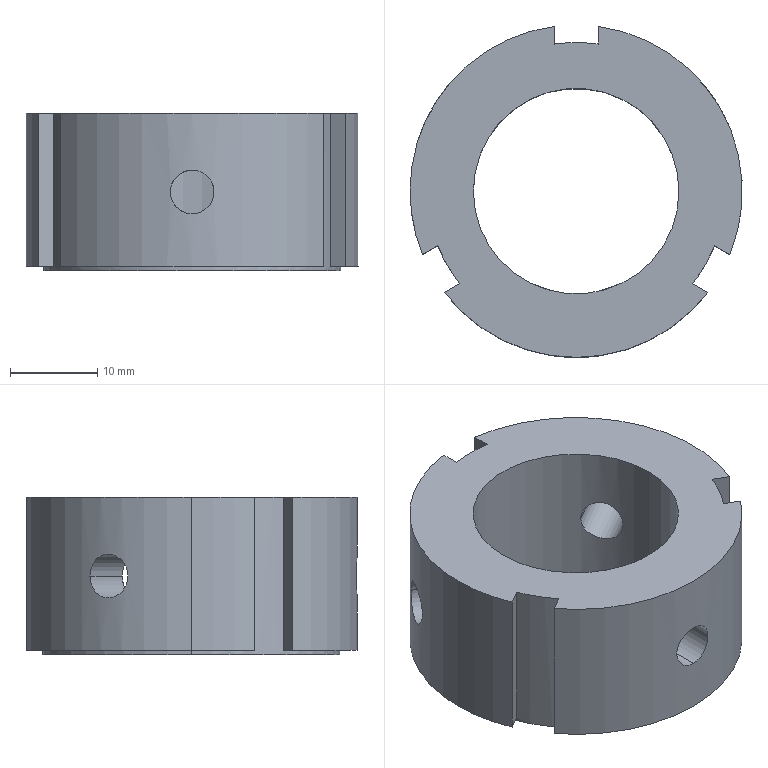Part | SolidWorks | features BaseBody 1 | 1 solid | 25 faces | box 38 x 37.835 x 18 mm | volume 11538 mm3 | cylinder 14 | plane 11 | commonest cylinder face diameters 5 x6 38 x4 23.5 x2 34 x2
STEP:
#1=CARTESIAN_POINT('',(0.,-11.75,6.5));
#2=VERTEX_POINT('',#1);
#3=CARTESIAN_POINT('',(0.,-11.75,11.5));
#4=VERTEX_POINT('',#3);
#5=CARTESIAN_POINT('',(0.,-11.75,6.5));
#6=CARTESIAN_POINT('',(-0.1656,-11.75,6.5));
#7=CARTESIAN_POINT('',(-0.3284,-11.747,6.516));
#8=CARTESIAN_POINT('',(-0.6485,-11.733,6.58));
#9=CARTESIAN_POINT('',(-0.8076,-11.723,6.628));
#10=CARTESIAN_POINT('',(-1.11,-11.698,6.754));
#11=CARTESIAN_POINT('',(-1.253,-11.684,6.831));
#12=CARTESIAN_POINT('',(-1.525,-11.651,7.012));
#13=CARTESIAN_POINT('',(-1.653,-11.634,7.117));
#14=CARTESIAN_POINT('',(-1.998,-11.581,7.462));
#15=CARTESIAN_POINT('',(-2.184,-11.546,7.74));
#16=CARTESIAN_POINT('',(-2.371,-11.508,8.191));
#17=CARTESIAN_POINT('',(-2.419,-11.498,8.349));
#18=CARTESIAN_POINT('',(-2.484,-11.485,8.672));
#19=CARTESIAN_POINT('',(-2.5,-11.481,8.834));
#20=CARTESIAN_POINT('',(-2.5,-11.481,9.161));
#21=CARTESIAN_POINT('',(-2.484,-11.485,9.328));
#22=CARTESIAN_POINT('',(-2.42,-11.498,9.649));
#23=CARTESIAN_POINT('',(-2.373,-11.508,9.805));
#24=CARTESIAN_POINT('',(-2.247,-11.533,10.108));
#25=CARTESIAN_POINT('',(-2.169,-11.548,10.254));
#26=CARTESIAN_POINT('',(-1.989,-11.581,10.524));
#27=CARTESIAN_POINT('',(-1.885,-11.598,10.651));
#28=CARTESIAN_POINT('',(-1.653,-11.634,10.883));
#29=CARTESIAN_POINT('',(-1.527,-11.651,10.986));
#30=CARTESIAN_POINT('',(-1.257,-11.683,11.167));
#31=CARTESIAN_POINT('',(-1.111,-11.698,11.246));
#32=CARTESIAN_POINT('',(-0.8086,-11.723,11.371));
#33=CARTESIAN_POINT('',(-0.6528,-11.733,11.419));
#34=CARTESIAN_POINT('',(-0.3315,-11.746,11.483));
#35=CARTESIAN_POINT('',(-0.1656,-11.75,11.5));
#36=CARTESIAN_POINT('',(0.,-11.75,11.5));
#37=B_SPLINE_CURVE_WITH_KNOTS('',3,(#5,#6,#7,#8,#9,#10,#11,#12,#13,#14,#15,#16,#17,#18,#19,#20,#21,#22,#23,#24,#25,#26,#27,#28,#29,#30,#31,#32,#33,#34,#35,#36),.UNSPECIFIED.,.F.,.F.,(4,2,2,2,2,2,2,2,2,2,2,2,2,2,2,4),(0.007836,0.008326,0.008816,0.009306,0.009795,0.01078,0.01126,0.01175,0.01224,0.01273,0.01322,0.01371,0.0142,0.01469,0.01518,0.01567),.UNSPECIFIED.);
#38=EDGE_CURVE('',#2,#4,#37,.T.);
#39=ORIENTED_EDGE('',*,*,#38,.F.);
#40=CARTESIAN_POINT('',(0.,-11.75,11.5));
#41=CARTESIAN_POINT('',(0.1656,-11.75,11.5));
#42=CARTESIAN_POINT('',(0.3284,-11.747,11.484));
#43=CARTESIAN_POINT('',(0.6485,-11.733,11.42));
#44=CARTESIAN_POINT('',(0.8076,-11.723,11.372));
#45=CARTESIAN_POINT('',(1.11,-11.698,11.246));
#46=CARTESIAN_POINT('',(1.253,-11.684,11.169));
#47=CARTESIAN_POINT('',(1.525,-11.651,10.988));
#48=CARTESIAN_POINT('',(1.653,-11.634,10.883));
#49=CARTESIAN_POINT('',(1.998,-11.581,10.538));
#50=CARTESIAN_POINT('',(2.184,-11.546,10.26));
#51=CARTESIAN_POINT('',(2.371,-11.508,9.809));
#52=CARTESIAN_POINT('',(2.419,-11.498,9.651));
#53=CARTESIAN_POINT('',(2.484,-11.485,9.328));
#54=CARTESIAN_POINT('',(2.5,-11.481,9.166));
#55=CARTESIAN_POINT('',(2.5,-11.481,8.839));
#56=CARTESIAN_POINT('',(2.484,-11.485,8.672));
#57=CARTESIAN_POINT('',(2.42,-11.498,8.351));
#58=CARTESIAN_POINT('',(2.373,-11.508,8.195));
#59=CARTESIAN_POINT('',(2.247,-11.533,7.892));
#60=CARTESIAN_POINT('',(2.169,-11.548,7.746));
#61=CARTESIAN_POINT('',(1.989,-11.581,7.476));
#62=CARTESIAN_POINT('',(1.885,-11.598,7.349));
#63=CARTESIAN_POINT('',(1.653,-11.634,7.117));
#64=CARTESIAN_POINT('',(1.527,-11.651,7.014));
#65=CARTESIAN_POINT('',(1.257,-11.683,6.833));
#66=CARTESIAN_POINT('',(1.111,-11.698,6.754));
#67=CARTESIAN_POINT('',(0.8086,-11.723,6.629));
#68=CARTESIAN_POINT('',(0.6528,-11.733,6.581));
#69=CARTESIAN_POINT('',(0.3315,-11.746,6.517));
#70=CARTESIAN_POINT('',(0.1656,-11.75,6.5));
#71=CARTESIAN_POINT('',(0.,-11.75,6.5));
#72=B_SPLINE_CURVE_WITH_KNOTS('',3,(#40,#41,#42,#43,#44,#45,#46,#47,#48,#49,#50,#51,#52,#53,#54,#55,#56,#57,#58,#59,#60,#61,#62,#63,#64,#65,#66,#67,#68,#69,#70,#71),.UNSPECIFIED.,.F.,.F.,(4,2,2,2,2,2,2,2,2,2,2,2,2,2,2,4),(0.,0.0004898,0.0009796,0.001469,0.001959,0.002939,0.003428,0.003918,0.004408,0.004898,0.005388,0.005877,0.006367,0.006857,0.007347,0.007836),.UNSPECIFIED.);
#73=EDGE_CURVE('',#4,#2,#72,.T.);
#74=ORIENTED_EDGE('',*,*,#73,.F.);
#75=EDGE_LOOP('',(#39,#74));
#76=FACE_BOUND('',#75,.T.);
#77=CARTESIAN_POINT('',(11.75,0.,18.));
#78=VERTEX_POINT('',#77);
#79=CARTESIAN_POINT('',(-11.75,0.,18.));
#80=VERTEX_POINT('',#79);
#81=CARTESIAN_POINT('',(0.,0.,18.));
#82=DIRECTION('',(0.,0.,-1.));
#83=DIRECTION('',(-1.,0.,0.));
#84=AXIS2_PLACEMENT_3D('',#81,#82,#83);
#85=CIRCLE('',#84,11.75);
#86=EDGE_CURVE('',#78,#80,#85,.T.);
#87=ORIENTED_EDGE('',*,*,#86,.F.);
#88=CARTESIAN_POINT('',(11.75,0.,0.));
#89=VERTEX_POINT('',#88);
#90=CARTESIAN_POINT('',(11.75,0.,18.));
#91=DIRECTION('',(0.,0.,-1.));
#92=VECTOR('',#91,1000.);
#93=LINE('',#90,#92);
#94=EDGE_CURVE('',#78,#89,#93,.T.);
#95=ORIENTED_EDGE('',*,*,#94,.T.);
#96=CARTESIAN_POINT('',(-11.75,0.,0.));
#97=VERTEX_POINT('',#96);
#98=CARTESIAN_POINT('',(0.,0.,0.));
#99=DIRECTION('',(0.,0.,1.));
#100=DIRECTION('',(-1.,0.,0.));
#101=AXIS2_PLACEMENT_3D('',#98,#99,#100);
#102=CIRCLE('',#101,11.75);
#103=EDGE_CURVE('',#97,#89,#102,.T.);
#104=ORIENTED_EDGE('',*,*,#103,.F.);
#105=CARTESIAN_POINT('',(-11.75,0.,18.));
#106=DIRECTION('',(0.,0.,-1.));
#107=VECTOR('',#106,1000.);
#108=LINE('',#105,#107);
#109=EDGE_CURVE('',#80,#97,#108,.T.);
#110=ORIENTED_EDGE('',*,*,#109,.F.);
#111=EDGE_LOOP('',(#87,#95,#104,#110));
#112=FACE_OUTER_BOUND('',#111,.T.);
#113=CARTESIAN_POINT('',(0.,0.,18.));
#114=DIRECTION('',(0.,0.,-1.));
#115=DIRECTION('',(-1.,0.,0.));
#116=AXIS2_PLACEMENT_3D('',#113,#114,#115);
#117=CYLINDRICAL_SURFACE('',#116,11.75);
#118=ADVANCED_FACE('',(#76,#112),#117,.F.);
#119=CARTESIAN_POINT('',(-19.,0.,18.));
#120=VERTEX_POINT('',#119);
#121=CARTESIAN_POINT('',(-17.561,-7.252,18.));
#122=VERTEX_POINT('',#121);
#123=CARTESIAN_POINT('',(0.,0.,18.));
#124=DIRECTION('',(0.,0.,1.));
#125=DIRECTION('',(-1.,0.,0.));
#126=AXIS2_PLACEMENT_3D('',#123,#124,#125);
#127=CIRCLE('',#126,19.);
#128=EDGE_CURVE('',#120,#122,#127,.T.);
#129=ORIENTED_EDGE('',*,*,#128,.F.);
#130=CARTESIAN_POINT('',(-19.,0.,0.5));
#131=VERTEX_POINT('',#130);
#132=CARTESIAN_POINT('',(-19.,0.,18.));
#133=DIRECTION('',(0.,0.,-1.));
#134=VECTOR('',#133,1000.);
#135=LINE('',#132,#134);
#136=EDGE_CURVE('',#120,#131,#135,.T.);
#137=ORIENTED_EDGE('',*,*,#136,.T.);
#138=CARTESIAN_POINT('',(-17.561,-7.252,0.5));
#139=VERTEX_POINT('',#138);
#140=CARTESIAN_POINT('',(0.,0.,0.5));
#141=DIRECTION('',(0.,0.,1.));
#142=DIRECTION('',(-1.,0.,0.));
#143=AXIS2_PLACEMENT_3D('',#140,#141,#142);
#144=CIRCLE('',#143,19.);
#145=EDGE_CURVE('',#131,#139,#144,.T.);
#146=ORIENTED_EDGE('',*,*,#145,.T.);
#147=CARTESIAN_POINT('',(-17.561,-7.252,18.));
#148=DIRECTION('',(0.,0.,1.));
#149=VECTOR('',#148,1000.);
#150=LINE('',#147,#149);
#151=EDGE_CURVE('',#139,#122,#150,.T.);
#152=ORIENTED_EDGE('',*,*,#151,.T.);
#153=EDGE_LOOP('',(#129,#137,#146,#152));
#154=FACE_OUTER_BOUND('',#153,.T.);
#155=CARTESIAN_POINT('',(0.,0.,18.));
#156=DIRECTION('',(0.,0.,-1.));
#157=DIRECTION('',(-1.,0.,0.));
#158=AXIS2_PLACEMENT_3D('',#155,#156,#157);
#159=CYLINDRICAL_SURFACE('',#158,19.);
#160=ADVANCED_FACE('',(#154),#159,.T.);
#161=CARTESIAN_POINT('',(2.5,16.815,0.5));
#162=VERTEX_POINT('',#161);
#163=CARTESIAN_POINT('',(17.,0.,0.5));
#164=VERTEX_POINT('',#163);
#165=CARTESIAN_POINT('',(0.,0.,0.5));
#166=DIRECTION('',(0.,0.,-1.));
#167=DIRECTION('',(-1.,0.,0.));
#168=AXIS2_PLACEMENT_3D('',#165,#166,#167);
#169=CIRCLE('',#168,17.);
#170=EDGE_CURVE('',#162,#164,#169,.T.);
#171=ORIENTED_EDGE('',*,*,#170,.T.);
#172=CARTESIAN_POINT('',(17.,0.,0.));
#173=VERTEX_POINT('',#172);
#174=CARTESIAN_POINT('',(17.,0.,0.5));
#175=DIRECTION('',(0.,0.,-1.));
#176=VECTOR('',#175,1000.);
#177=LINE('',#174,#176);
#178=EDGE_CURVE('',#164,#173,#177,.T.);
#179=ORIENTED_EDGE('',*,*,#178,.T.);
#180=CARTESIAN_POINT('',(-17.,0.,0.));
#181=VERTEX_POINT('',#180);
#182=CARTESIAN_POINT('',(0.,0.,0.));
#183=DIRECTION('',(0.,0.,1.));
#184=DIRECTION('',(-1.,0.,0.));
#185=AXIS2_PLACEMENT_3D('',#182,#183,#184);
#186=CIRCLE('',#185,17.);
#187=EDGE_CURVE('',#173,#181,#186,.T.);
#188=ORIENTED_EDGE('',*,*,#187,.T.);
#189=CARTESIAN_POINT('',(-17.,0.,0.5));
#190=VERTEX_POINT('',#189);
#191=CARTESIAN_POINT('',(-17.,0.,0.5));
#192=DIRECTION('',(0.,0.,-1.));
#193=VECTOR('',#192,1000.);
#194=LINE('',#191,#193);
#195=EDGE_CURVE('',#190,#181,#194,.T.);
#196=ORIENTED_EDGE('',*,*,#195,.F.);
#197=CARTESIAN_POINT('',(-2.5,16.815,0.5));
#198=VERTEX_POINT('',#197);
#199=CARTESIAN_POINT('',(0.,0.,0.5));
#200=DIRECTION('',(0.,0.,-1.));
#201=DIRECTION('',(-1.,0.,0.));
#202=AXIS2_PLACEMENT_3D('',#199,#200,#201);
#203=CIRCLE('',#202,17.);
#204=EDGE_CURVE('',#190,#198,#203,.T.);
#205=ORIENTED_EDGE('',*,*,#204,.T.);
#206=CARTESIAN_POINT('',(-2.5,16.815,18.));
#207=VERTEX_POINT('',#206);
#208=CARTESIAN_POINT('',(-2.5,16.815,18.));
#209=DIRECTION('',(0.,0.,1.));
#210=VECTOR('',#209,1000.);
#211=LINE('',#208,#210);
#212=EDGE_CURVE('',#198,#207,#211,.T.);
#213=ORIENTED_EDGE('',*,*,#212,.T.);
#214=CARTESIAN_POINT('',(2.5,16.815,18.));
#215=VERTEX_POINT('',#214);
#216=CARTESIAN_POINT('',(0.,0.,18.));
#217=DIRECTION('',(0.,0.,1.));
#218=DIRECTION('',(-1.,0.,0.));
#219=AXIS2_PLACEMENT_3D('',#216,#217,#218);
#220=CIRCLE('',#219,17.);
#221=EDGE_CURVE('',#215,#207,#220,.T.);
#222=ORIENTED_EDGE('',*,*,#221,.F.);
#223=CARTESIAN_POINT('',(2.5,16.815,0.5));
#224=DIRECTION('',(0.,0.,-1.));
#225=VECTOR('',#224,1000.);
#226=LINE('',#223,#225);
#227=EDGE_CURVE('',#215,#162,#226,.T.);
#228=ORIENTED_EDGE('',*,*,#227,.T.);
#229=EDGE_LOOP('',(#171,#179,#188,#196,#205,#213,#222,#228));
#230=FACE_OUTER_BOUND('',#229,.T.);
#231=CARTESIAN_POINT('',(0.,0.,0.5));
#232=DIRECTION('',(0.,0.,-1.));
#233=DIRECTION('',(-1.,0.,0.));
#234=AXIS2_PLACEMENT_3D('',#231,#232,#233);
#235=CYLINDRICAL_SURFACE('',#234,17.);
#236=ADVANCED_FACE('',(#230),#235,.T.);
#237=ORIENTED_EDGE('',*,*,#38,.T.);
#238=CARTESIAN_POINT('',(0.,-19.,11.5));
#239=VERTEX_POINT('',#238);
#240=CARTESIAN_POINT('',(0.,-19.,11.5));
#241=DIRECTION('',(0.,-1.,0.));
#242=VECTOR('',#241,1000.);
#243=LINE('',#240,#242);
#244=EDGE_CURVE('',#4,#239,#243,.T.);
#245=ORIENTED_EDGE('',*,*,#244,.T.);
#246=CARTESIAN_POINT('',(0.,-19.,6.5));
#247=VERTEX_POINT('',#246);
#248=CARTESIAN_POINT('',(0.,-19.,6.5));
#249=CARTESIAN_POINT('',(-0.1653,-19.,6.5));
#250=CARTESIAN_POINT('',(-0.3279,-18.998,6.516));
#251=CARTESIAN_POINT('',(-0.6476,-18.99,6.58));
#252=CARTESIAN_POINT('',(-0.8064,-18.983,6.628));
#253=CARTESIAN_POINT('',(-1.109,-18.968,6.753));
#254=CARTESIAN_POINT('',(-1.253,-18.959,6.83));
#255=CARTESIAN_POINT('',(-1.524,-18.939,7.012));
#256=CARTESIAN_POINT('',(-1.653,-18.928,7.117));
#257=CARTESIAN_POINT('',(-1.883,-18.907,7.347));
#258=CARTESIAN_POINT('',(-1.986,-18.896,7.473));
#259=CARTESIAN_POINT('',(-2.169,-18.876,7.746));
#260=CARTESIAN_POINT('',(-2.247,-18.867,7.892));
#261=CARTESIAN_POINT('',(-2.371,-18.852,8.192));
#262=CARTESIAN_POINT('',(-2.42,-18.845,8.35));
#263=CARTESIAN_POINT('',(-2.484,-18.837,8.673));
#264=CARTESIAN_POINT('',(-2.5,-18.835,8.835));
#265=CARTESIAN_POINT('',(-2.5,-18.835,9.161));
#266=CARTESIAN_POINT('',(-2.484,-18.837,9.327));
#267=CARTESIAN_POINT('',(-2.42,-18.845,9.648));
#268=CARTESIAN_POINT('',(-2.373,-18.851,9.804));
#269=CARTESIAN_POINT('',(-2.248,-18.867,10.107));
#270=CARTESIAN_POINT('',(-2.17,-18.876,10.253));
#271=CARTESIAN_POINT('',(-1.989,-18.896,10.524));
#272=CARTESIAN_POINT('',(-1.885,-18.907,10.65));
#273=CARTESIAN_POINT('',(-1.652,-18.928,10.883));
#274=CARTESIAN_POINT('',(-1.526,-18.939,10.987));
#275=CARTESIAN_POINT('',(-1.256,-18.959,11.168));
#276=CARTESIAN_POINT('',(-1.11,-18.968,11.246));
#277=CARTESIAN_POINT('',(-0.8072,-18.983,11.372));
#278=CARTESIAN_POINT('',(-0.6515,-18.99,11.419));
#279=CARTESIAN_POINT('',(-0.3308,-18.998,11.483));
#280=CARTESIAN_POINT('',(-0.1653,-19.,11.5));
#281=CARTESIAN_POINT('',(0.,-19.,11.5));
#282=B_SPLINE_CURVE_WITH_KNOTS('',3,(#248,#249,#250,#251,#252,#253,#254,#255,#256,#257,#258,#259,#260,#261,#262,#263,#264,#265,#266,#267,#268,#269,#270,#271,#272,#273,#274,#275,#276,#277,#278,#279,#280,#281),.UNSPECIFIED.,.F.,.F.,(4,2,2,2,2,2,2,2,2,2,2,2,2,2,2,2,4),(0.007823,0.008312,0.008801,0.00929,0.009779,0.01027,0.01076,0.01125,0.01173,0.01222,0.01271,0.0132,0.01369,0.01418,0.01467,0.01516,0.01565),.UNSPECIFIED.);
#283=EDGE_CURVE('',#247,#239,#282,.T.);
#284=ORIENTED_EDGE('',*,*,#283,.F.);
#285=CARTESIAN_POINT('',(0.,-19.,6.5));
#286=DIRECTION('',(0.,-1.,0.));
#287=VECTOR('',#286,1000.);
#288=LINE('',#285,#287);
#289=EDGE_CURVE('',#2,#247,#288,.T.);
#290=ORIENTED_EDGE('',*,*,#289,.F.);
#291=EDGE_LOOP('',(#237,#245,#284,#290));
#292=FACE_OUTER_BOUND('',#291,.T.);
#293=CARTESIAN_POINT('',(0.,-19.,9.));
#294=DIRECTION('',(0.,-1.,0.));
#295=DIRECTION('',(0.,0.,-1.));
#296=AXIS2_PLACEMENT_3D('',#293,#294,#295);
#297=CYLINDRICAL_SURFACE('',#296,2.5);
#298=ADVANCED_FACE('',(#292),#297,.F.);
#299=CARTESIAN_POINT('',(8.693,7.906,9.));
#300=VERTEX_POINT('',#299);
#301=CARTESIAN_POINT('',(11.193,3.575,9.));
#302=VERTEX_POINT('',#301);
#303=CARTESIAN_POINT('',(8.693,7.906,9.));
#304=CARTESIAN_POINT('',(8.693,7.906,8.836));
#305=CARTESIAN_POINT('',(8.704,7.893,8.67));
#306=CARTESIAN_POINT('',(8.748,7.844,8.349));
#307=CARTESIAN_POINT('',(8.78,7.808,8.193));
#308=CARTESIAN_POINT('',(8.865,7.712,7.89));
#309=CARTESIAN_POINT('',(8.917,7.652,7.745));
#310=CARTESIAN_POINT('',(9.036,7.512,7.474));
#311=CARTESIAN_POINT('',(9.103,7.43,7.348));
#312=CARTESIAN_POINT('',(9.25,7.247,7.116));
#313=CARTESIAN_POINT('',(9.328,7.147,7.013));
#314=CARTESIAN_POINT('',(9.491,6.929,6.832));
#315=CARTESIAN_POINT('',(9.577,6.809,6.753));
#316=CARTESIAN_POINT('',(9.749,6.56,6.628));
#317=CARTESIAN_POINT('',(9.836,6.43,6.581));
#318=CARTESIAN_POINT('',(10.008,6.159,6.516));
#319=CARTESIAN_POINT('',(10.094,6.017,6.5));
#320=CARTESIAN_POINT('',(10.26,5.73,6.5));
#321=CARTESIAN_POINT('',(10.338,5.587,6.517));
#322=CARTESIAN_POINT('',(10.486,5.303,6.581));
#323=CARTESIAN_POINT('',(10.557,5.16,6.629));
#324=CARTESIAN_POINT('',(10.687,4.886,6.755));
#325=CARTESIAN_POINT('',(10.746,4.755,6.832));
#326=CARTESIAN_POINT('',(10.853,4.504,7.013));
#327=CARTESIAN_POINT('',(10.902,4.384,7.119));
#328=CARTESIAN_POINT('',(11.029,4.059,7.464));
#329=CARTESIAN_POINT('',(11.091,3.881,7.742));
#330=CARTESIAN_POINT('',(11.152,3.7,8.193));
#331=CARTESIAN_POINT('',(11.168,3.653,8.351));
#332=CARTESIAN_POINT('',(11.188,3.591,8.674));
#333=CARTESIAN_POINT('',(11.193,3.575,8.836));
#334=CARTESIAN_POINT('',(11.193,3.575,9.));
#335=B_SPLINE_CURVE_WITH_KNOTS('',3,(#303,#304,#305,#306,#307,#308,#309,#310,#311,#312,#313,#314,#315,#316,#317,#318,#319,#320,#321,#322,#323,#324,#325,#326,#327,#328,#329,#330,#331,#332,#333,#334),.UNSPECIFIED.,.F.,.F.,(4,2,2,2,2,2,2,2,2,2,2,2,2,2,2,4),(0.00392,0.00441,0.0049,0.00539,0.005879,0.006369,0.006859,0.007349,0.007838,0.008328,0.008818,0.009308,0.009798,0.01078,0.01127,0.01176),.UNSPECIFIED.);
#336=EDGE_CURVE('',#300,#302,#335,.T.);
#337=ORIENTED_EDGE('',*,*,#336,.T.);
#338=CARTESIAN_POINT('',(17.561,7.252,9.));
#339=VERTEX_POINT('',#338);
#340=CARTESIAN_POINT('',(17.704,7.335,9.));
#341=DIRECTION('',(0.866,0.5,0.));
#342=VECTOR('',#341,1000.);
#343=LINE('',#340,#342);
#344=EDGE_CURVE('',#302,#339,#343,.T.);
#345=ORIENTED_EDGE('',*,*,#344,.T.);
#346=CARTESIAN_POINT('',(15.061,11.582,9.));
#347=VERTEX_POINT('',#346);
#348=CARTESIAN_POINT('',(15.061,11.582,9.));
#349=CARTESIAN_POINT('',(15.061,11.582,8.837));
#350=CARTESIAN_POINT('',(15.072,11.569,8.671));
#351=CARTESIAN_POINT('',(15.111,11.518,8.35));
#352=CARTESIAN_POINT('',(15.14,11.48,8.194));
#353=CARTESIAN_POINT('',(15.216,11.379,7.892));
#354=CARTESIAN_POINT('',(15.263,11.316,7.746));
#355=CARTESIAN_POINT('',(15.371,11.169,7.475));
#356=CARTESIAN_POINT('',(15.432,11.085,7.349));
#357=CARTESIAN_POINT('',(15.567,10.894,7.116));
#358=CARTESIAN_POINT('',(15.639,10.79,7.012));
#359=CARTESIAN_POINT('',(15.792,10.566,6.831));
#360=CARTESIAN_POINT('',(15.873,10.444,6.753));
#361=CARTESIAN_POINT('',(16.037,10.189,6.628));
#362=CARTESIAN_POINT('',(16.121,10.057,6.58));
#363=CARTESIAN_POINT('',(16.288,9.784,6.516));
#364=CARTESIAN_POINT('',(16.373,9.642,6.5));
#365=CARTESIAN_POINT('',(16.538,9.355,6.5));
#366=CARTESIAN_POINT('',(16.617,9.213,6.516));
#367=CARTESIAN_POINT('',(16.77,8.932,6.58));
#368=CARTESIAN_POINT('',(16.844,8.792,6.629));
#369=CARTESIAN_POINT('',(16.982,8.522,6.754));
#370=CARTESIAN_POINT('',(17.046,8.393,6.831));
#371=CARTESIAN_POINT('',(17.165,8.148,7.013));
#372=CARTESIAN_POINT('',(17.219,8.032,7.118));
#373=CARTESIAN_POINT('',(17.316,7.822,7.349));
#374=CARTESIAN_POINT('',(17.358,7.727,7.475));
#375=CARTESIAN_POINT('',(17.432,7.559,7.748));
#376=CARTESIAN_POINT('',(17.463,7.487,7.893));
#377=CARTESIAN_POINT('',(17.512,7.371,8.194));
#378=CARTESIAN_POINT('',(17.531,7.327,8.352));
#379=CARTESIAN_POINT('',(17.555,7.267,8.674));
#380=CARTESIAN_POINT('',(17.561,7.252,8.837));
#381=CARTESIAN_POINT('',(17.561,7.252,9.));
#382=B_SPLINE_CURVE_WITH_KNOTS('',3,(#348,#349,#350,#351,#352,#353,#354,#355,#356,#357,#358,#359,#360,#361,#362,#363,#364,#365,#366,#367,#368,#369,#370,#371,#372,#373,#374,#375,#376,#377,#378,#379,#380,#381),.UNSPECIFIED.,.F.,.F.,(4,2,2,2,2,2,2,2,2,2,2,2,2,2,2,2,4),(0.003913,0.004402,0.004891,0.00538,0.005869,0.006358,0.006847,0.007336,0.007825,0.008314,0.008802,0.009291,0.00978,0.01027,0.01076,0.01125,0.01174),.UNSPECIFIED.);
#383=EDGE_CURVE('',#347,#339,#382,.T.);
#384=ORIENTED_EDGE('',*,*,#383,.F.);
#385=CARTESIAN_POINT('',(15.204,11.665,9.));
#386=DIRECTION('',(0.866,0.5,0.));
#387=VECTOR('',#386,1000.);
#388=LINE('',#385,#387);
#389=EDGE_CURVE('',#300,#347,#388,.T.);
#390=ORIENTED_EDGE('',*,*,#389,.F.);
#391=EDGE_LOOP('',(#337,#345,#384,#390));
#392=FACE_OUTER_BOUND('',#391,.T.);
#393=CARTESIAN_POINT('',(16.454,9.5,9.));
#394=DIRECTION('',(0.866,0.5,0.));
#395=DIRECTION('',(-0.5,0.866,0.));
#396=AXIS2_PLACEMENT_3D('',#393,#394,#395);
#397=CYLINDRICAL_SURFACE('',#396,2.5);
#398=ADVANCED_FACE('',(#392),#397,.F.);
#399=CARTESIAN_POINT('',(-11.193,3.575,9.));
#400=VERTEX_POINT('',#399);
#401=CARTESIAN_POINT('',(-8.693,7.906,9.));
#402=VERTEX_POINT('',#401);
#403=CARTESIAN_POINT('',(-11.193,3.575,9.));
#404=CARTESIAN_POINT('',(-11.193,3.575,8.836));
#405=CARTESIAN_POINT('',(-11.188,3.591,8.67));
#406=CARTESIAN_POINT('',(-11.167,3.654,8.349));
#407=CARTESIAN_POINT('',(-11.152,3.7,8.193));
#408=CARTESIAN_POINT('',(-11.111,3.821,7.89));
#409=CARTESIAN_POINT('',(-11.085,3.897,7.745));
#410=CARTESIAN_POINT('',(-11.023,4.07,7.474));
#411=CARTESIAN_POINT('',(-10.986,4.168,7.348));
#412=CARTESIAN_POINT('',(-10.901,4.387,7.116));
#413=CARTESIAN_POINT('',(-10.853,4.505,7.013));
#414=CARTESIAN_POINT('',(-10.746,4.755,6.832));
#415=CARTESIAN_POINT('',(-10.686,4.889,6.753));
#416=CARTESIAN_POINT('',(-10.556,5.163,6.628));
#417=CARTESIAN_POINT('',(-10.487,5.303,6.581));
#418=CARTESIAN_POINT('',(-10.337,5.588,6.516));
#419=CARTESIAN_POINT('',(-10.258,5.733,6.5));
#420=CARTESIAN_POINT('',(-10.092,6.02,6.5));
#421=CARTESIAN_POINT('',(-10.007,6.159,6.517));
#422=CARTESIAN_POINT('',(-9.836,6.43,6.581));
#423=CARTESIAN_POINT('',(-9.748,6.563,6.629));
#424=CARTESIAN_POINT('',(-9.575,6.812,6.755));
#425=CARTESIAN_POINT('',(-9.491,6.929,6.832));
#426=CARTESIAN_POINT('',(-9.327,7.148,7.013));
#427=CARTESIAN_POINT('',(-9.248,7.25,7.119));
#428=CARTESIAN_POINT('',(-9.03,7.522,7.464));
#429=CARTESIAN_POINT('',(-8.907,7.665,7.742));
#430=CARTESIAN_POINT('',(-8.781,7.808,8.193));
#431=CARTESIAN_POINT('',(-8.748,7.845,8.351));
#432=CARTESIAN_POINT('',(-8.704,7.894,8.674));
#433=CARTESIAN_POINT('',(-8.693,7.906,8.836));
#434=CARTESIAN_POINT('',(-8.693,7.906,9.));
#435=B_SPLINE_CURVE_WITH_KNOTS('',3,(#403,#404,#405,#406,#407,#408,#409,#410,#411,#412,#413,#414,#415,#416,#417,#418,#419,#420,#421,#422,#423,#424,#425,#426,#427,#428,#429,#430,#431,#432,#433,#434),.UNSPECIFIED.,.F.,.F.,(4,2,2,2,2,2,2,2,2,2,2,2,2,2,2,4),(0.00392,0.00441,0.0049,0.00539,0.005879,0.006369,0.006859,0.007349,0.007838,0.008328,0.008818,0.009308,0.009798,0.01078,0.01127,0.01176),.UNSPECIFIED.);
#436=EDGE_CURVE('',#400,#402,#435,.T.);
#437=ORIENTED_EDGE('',*,*,#436,.T.);
#438=CARTESIAN_POINT('',(-15.061,11.582,9.));
#439=VERTEX_POINT('',#438);
#440=CARTESIAN_POINT('',(-15.204,11.665,9.));
#441=DIRECTION('',(-0.866,0.5,0.));
#442=VECTOR('',#441,1000.);
#443=LINE('',#440,#442);
#444=EDGE_CURVE('',#402,#439,#443,.T.);
#445=ORIENTED_EDGE('',*,*,#444,.T.);
#446=CARTESIAN_POINT('',(-17.561,7.252,9.));
#447=VERTEX_POINT('',#446);
#448=CARTESIAN_POINT('',(-17.561,7.252,9.));
#449=CARTESIAN_POINT('',(-17.561,7.252,8.837));
#450=CARTESIAN_POINT('',(-17.555,7.268,8.671));
#451=CARTESIAN_POINT('',(-17.53,7.327,8.35));
#452=CARTESIAN_POINT('',(-17.512,7.371,8.194));
#453=CARTESIAN_POINT('',(-17.463,7.488,7.892));
#454=CARTESIAN_POINT('',(-17.431,7.56,7.746));
#455=CARTESIAN_POINT('',(-17.358,7.727,7.475));
#456=CARTESIAN_POINT('',(-17.316,7.822,7.349));
#457=CARTESIAN_POINT('',(-17.218,8.034,7.116));
#458=CARTESIAN_POINT('',(-17.164,8.149,7.012));
#459=CARTESIAN_POINT('',(-17.046,8.393,6.831));
#460=CARTESIAN_POINT('',(-16.981,8.524,6.753));
#461=CARTESIAN_POINT('',(-16.843,8.794,6.628));
#462=CARTESIAN_POINT('',(-16.77,8.932,6.58));
#463=CARTESIAN_POINT('',(-16.617,9.214,6.516));
#464=CARTESIAN_POINT('',(-16.536,9.358,6.5));
#465=CARTESIAN_POINT('',(-16.371,9.645,6.5));
#466=CARTESIAN_POINT('',(-16.288,9.784,6.516));
#467=CARTESIAN_POINT('',(-16.121,10.057,6.58));
#468=CARTESIAN_POINT('',(-16.036,10.192,6.629));
#469=CARTESIAN_POINT('',(-15.872,10.446,6.754));
#470=CARTESIAN_POINT('',(-15.792,10.566,6.831));
#471=CARTESIAN_POINT('',(-15.639,10.791,7.013));
#472=CARTESIAN_POINT('',(-15.565,10.897,7.118));
#473=CARTESIAN_POINT('',(-15.432,11.085,7.349));
#474=CARTESIAN_POINT('',(-15.371,11.169,7.475));
#475=CARTESIAN_POINT('',(-15.262,11.317,7.748));
#476=CARTESIAN_POINT('',(-15.215,11.38,7.893));
#477=CARTESIAN_POINT('',(-15.14,11.48,8.194));
#478=CARTESIAN_POINT('',(-15.11,11.518,8.352));
#479=CARTESIAN_POINT('',(-15.071,11.57,8.674));
#480=CARTESIAN_POINT('',(-15.061,11.582,8.837));
#481=CARTESIAN_POINT('',(-15.061,11.582,9.));
#482=B_SPLINE_CURVE_WITH_KNOTS('',3,(#448,#449,#450,#451,#452,#453,#454,#455,#456,#457,#458,#459,#460,#461,#462,#463,#464,#465,#466,#467,#468,#469,#470,#471,#472,#473,#474,#475,#476,#477,#478,#479,#480,#481),.UNSPECIFIED.,.F.,.F.,(4,2,2,2,2,2,2,2,2,2,2,2,2,2,2,2,4),(0.003913,0.004402,0.004891,0.00538,0.005869,0.006358,0.006847,0.007336,0.007825,0.008314,0.008802,0.009291,0.00978,0.01027,0.01076,0.01125,0.01174),.UNSPECIFIED.);
#483=EDGE_CURVE('',#447,#439,#482,.T.);
#484=ORIENTED_EDGE('',*,*,#483,.F.);
#485=CARTESIAN_POINT('',(-17.704,7.335,9.));
#486=DIRECTION('',(-0.866,0.5,0.));
#487=VECTOR('',#486,1000.);
#488=LINE('',#485,#487);
#489=EDGE_CURVE('',#400,#447,#488,.T.);
#490=ORIENTED_EDGE('',*,*,#489,.F.);
#491=EDGE_LOOP('',(#437,#445,#484,#490));
#492=FACE_OUTER_BOUND('',#491,.T.);
#493=CARTESIAN_POINT('',(-16.454,9.5,9.));
#494=DIRECTION('',(-0.866,0.5,0.));
#495=DIRECTION('',(-0.5,-0.866,0.));
#496=AXIS2_PLACEMENT_3D('',#493,#494,#495);
#497=CYLINDRICAL_SURFACE('',#496,2.5);
#498=ADVANCED_FACE('',(#492),#497,.F.);
#499=CARTESIAN_POINT('',(0.,0.,18.));
#500=DIRECTION('',(0.,0.,-1.));
#501=DIRECTION('',(-1.,0.,0.));
#502=AXIS2_PLACEMENT_3D('',#499,#500,#501);
#503=CIRCLE('',#502,11.75);
#504=EDGE_CURVE('',#80,#78,#503,.T.);
#505=ORIENTED_EDGE('',*,*,#504,.T.);
#506=ORIENTED_EDGE('',*,*,#86,.T.);
#507=EDGE_LOOP('',(#505,#506));
#508=FACE_BOUND('',#507,.T.);
#509=CARTESIAN_POINT('',(-2.5,18.835,18.));
#510=VERTEX_POINT('',#509);
#511=CARTESIAN_POINT('',(0.,0.,18.));
#512=DIRECTION('',(0.,0.,1.));
#513=DIRECTION('',(-1.,0.,0.));
#514=AXIS2_PLACEMENT_3D('',#511,#512,#513);
#515=CIRCLE('',#514,19.);
#516=EDGE_CURVE('',#510,#120,#515,.T.);
#517=ORIENTED_EDGE('',*,*,#516,.T.);
#518=ORIENTED_EDGE('',*,*,#128,.T.);
#519=CARTESIAN_POINT('',(-15.812,-6.243,18.));
#520=VERTEX_POINT('',#519);
#521=CARTESIAN_POINT('',(-17.561,-7.252,18.));
#522=DIRECTION('',(0.866,0.5,0.));
#523=VECTOR('',#522,1000.);
#524=LINE('',#521,#523);
#525=EDGE_CURVE('',#122,#520,#524,.T.);
#526=ORIENTED_EDGE('',*,*,#525,.T.);
#527=CARTESIAN_POINT('',(-13.312,-10.573,18.));
#528=VERTEX_POINT('',#527);
#529=CARTESIAN_POINT('',(0.,0.,18.));
#530=DIRECTION('',(0.,0.,1.));
#531=DIRECTION('',(-1.,0.,0.));
#532=AXIS2_PLACEMENT_3D('',#529,#530,#531);
#533=CIRCLE('',#532,17.);
#534=EDGE_CURVE('',#520,#528,#533,.T.);
#535=ORIENTED_EDGE('',*,*,#534,.T.);
#536=CARTESIAN_POINT('',(-15.061,-11.582,18.));
#537=VERTEX_POINT('',#536);
#538=CARTESIAN_POINT('',(-13.312,-10.573,18.));
#539=DIRECTION('',(-0.866,-0.5,0.));
#540=VECTOR('',#539,1000.);
#541=LINE('',#538,#540);
#542=EDGE_CURVE('',#528,#537,#541,.T.);
#543=ORIENTED_EDGE('',*,*,#542,.T.);
#544=CARTESIAN_POINT('',(15.061,-11.582,18.));
#545=VERTEX_POINT('',#544);
#546=CARTESIAN_POINT('',(0.,0.,18.));
#547=DIRECTION('',(0.,0.,1.));
#548=DIRECTION('',(-1.,0.,0.));
#549=AXIS2_PLACEMENT_3D('',#546,#547,#548);
#550=CIRCLE('',#549,19.);
#551=EDGE_CURVE('',#537,#545,#550,.T.);
#552=ORIENTED_EDGE('',*,*,#551,.T.);
#553=CARTESIAN_POINT('',(13.312,-10.573,18.));
#554=VERTEX_POINT('',#553);
#555=CARTESIAN_POINT('',(15.061,-11.582,18.));
#556=DIRECTION('',(-0.866,0.5,0.));
#557=VECTOR('',#556,1000.);
#558=LINE('',#555,#557);
#559=EDGE_CURVE('',#545,#554,#558,.T.);
#560=ORIENTED_EDGE('',*,*,#559,.T.);
#561=CARTESIAN_POINT('',(15.812,-6.243,18.));
#562=VERTEX_POINT('',#561);
#563=CARTESIAN_POINT('',(0.,0.,18.));
#564=DIRECTION('',(0.,0.,1.));
#565=DIRECTION('',(-1.,0.,0.));
#566=AXIS2_PLACEMENT_3D('',#563,#564,#565);
#567=CIRCLE('',#566,17.);
#568=EDGE_CURVE('',#554,#562,#567,.T.);
#569=ORIENTED_EDGE('',*,*,#568,.T.);
#570=CARTESIAN_POINT('',(17.561,-7.252,18.));
#571=VERTEX_POINT('',#570);
#572=CARTESIAN_POINT('',(15.812,-6.243,18.));
#573=DIRECTION('',(0.866,-0.5,0.));
#574=VECTOR('',#573,1000.);
#575=LINE('',#572,#574);
#576=EDGE_CURVE('',#562,#571,#575,.T.);
#577=ORIENTED_EDGE('',*,*,#576,.T.);
#578=CARTESIAN_POINT('',(2.5,18.835,18.));
#579=VERTEX_POINT('',#578);
#580=CARTESIAN_POINT('',(0.,0.,18.));
#581=DIRECTION('',(0.,0.,1.));
#582=DIRECTION('',(-1.,0.,0.));
#583=AXIS2_PLACEMENT_3D('',#580,#581,#582);
#584=CIRCLE('',#583,19.);
#585=EDGE_CURVE('',#571,#579,#584,.T.);
#586=ORIENTED_EDGE('',*,*,#585,.T.);
#587=CARTESIAN_POINT('',(2.5,0.,18.));
#588=DIRECTION('',(0.,-1.,0.));
#589=VECTOR('',#588,1000.);
#590=LINE('',#587,#589);
#591=EDGE_CURVE('',#579,#215,#590,.T.);
#592=ORIENTED_EDGE('',*,*,#591,.T.);
#593=ORIENTED_EDGE('',*,*,#221,.T.);
#594=CARTESIAN_POINT('',(-2.5,0.,18.));
#595=DIRECTION('',(0.,1.,0.));
#596=VECTOR('',#595,1000.);
#597=LINE('',#594,#596);
#598=EDGE_CURVE('',#207,#510,#597,.T.);
#599=ORIENTED_EDGE('',*,*,#598,.T.);
#600=EDGE_LOOP('',(#517,#518,#526,#535,#543,#552,#560,#569,#577,#586,#592,#593,#599));
#601=FACE_OUTER_BOUND('',#600,.T.);
#602=CARTESIAN_POINT('',(0.,0.,18.));
#603=DIRECTION('',(0.,0.,1.));
#604=DIRECTION('',(1.,0.,0.));
#605=AXIS2_PLACEMENT_3D('',#602,#603,#604);
#606=PLANE('',#605);
#607=ADVANCED_FACE('',(#508,#601),#606,.T.);
#608=ORIENTED_EDGE('',*,*,#94,.F.);
#609=ORIENTED_EDGE('',*,*,#504,.F.);
#610=ORIENTED_EDGE('',*,*,#109,.T.);
#611=CARTESIAN_POINT('',(0.,0.,0.));
#612=DIRECTION('',(0.,0.,1.));
#613=DIRECTION('',(-1.,0.,0.));
#614=AXIS2_PLACEMENT_3D('',#611,#612,#613);
#615=CIRCLE('',#614,11.75);
#616=EDGE_CURVE('',#89,#97,#615,.T.);
#617=ORIENTED_EDGE('',*,*,#616,.F.);
#618=EDGE_LOOP('',(#608,#609,#610,#617));
#619=FACE_OUTER_BOUND('',#618,.T.);
#620=ORIENTED_EDGE('',*,*,#336,.F.);
#621=CARTESIAN_POINT('',(11.193,3.575,9.));
#622=CARTESIAN_POINT('',(11.193,3.575,9.164));
#623=CARTESIAN_POINT('',(11.188,3.591,9.33));
#624=CARTESIAN_POINT('',(11.167,3.654,9.651));
#625=CARTESIAN_POINT('',(11.152,3.7,9.807));
#626=CARTESIAN_POINT('',(11.111,3.821,10.11));
#627=CARTESIAN_POINT('',(11.085,3.897,10.255));
#628=CARTESIAN_POINT('',(11.023,4.07,10.526));
#629=CARTESIAN_POINT('',(10.986,4.168,10.652));
#630=CARTESIAN_POINT('',(10.901,4.387,10.884));
#631=CARTESIAN_POINT('',(10.853,4.505,10.987));
#632=CARTESIAN_POINT('',(10.746,4.755,11.168));
#633=CARTESIAN_POINT('',(10.686,4.889,11.247));
#634=CARTESIAN_POINT('',(10.556,5.163,11.372));
#635=CARTESIAN_POINT('',(10.487,5.303,11.419));
#636=CARTESIAN_POINT('',(10.337,5.588,11.484));
#637=CARTESIAN_POINT('',(10.258,5.733,11.5));
#638=CARTESIAN_POINT('',(10.092,6.02,11.5));
#639=CARTESIAN_POINT('',(10.007,6.159,11.483));
#640=CARTESIAN_POINT('',(9.836,6.43,11.419));
#641=CARTESIAN_POINT('',(9.748,6.563,11.371));
#642=CARTESIAN_POINT('',(9.575,6.812,11.245));
#643=CARTESIAN_POINT('',(9.491,6.929,11.168));
#644=CARTESIAN_POINT('',(9.327,7.148,10.987));
#645=CARTESIAN_POINT('',(9.248,7.25,10.881));
#646=CARTESIAN_POINT('',(9.03,7.522,10.536));
#647=CARTESIAN_POINT('',(8.907,7.665,10.258));
#648=CARTESIAN_POINT('',(8.781,7.808,9.807));
#649=CARTESIAN_POINT('',(8.748,7.845,9.649));
#650=CARTESIAN_POINT('',(8.704,7.894,9.326));
#651=CARTESIAN_POINT('',(8.693,7.906,9.164));
#652=CARTESIAN_POINT('',(8.693,7.906,9.));
#653=B_SPLINE_CURVE_WITH_KNOTS('',3,(#621,#622,#623,#624,#625,#626,#627,#628,#629,#630,#631,#632,#633,#634,#635,#636,#637,#638,#639,#640,#641,#642,#643,#644,#645,#646,#647,#648,#649,#650,#651,#652),.UNSPECIFIED.,.F.,.F.,(4,2,2,2,2,2,2,2,2,2,2,2,2,2,2,4),(0.01176,0.01225,0.01274,0.01323,0.01372,0.01421,0.0147,0.01519,0.01567,0.01616,0.01665,0.01714,0.01763,0.01861,0.0191,0.01959),.UNSPECIFIED.);
#654=EDGE_CURVE('',#302,#300,#653,.T.);
#655=ORIENTED_EDGE('',*,*,#654,.F.);
#656=EDGE_LOOP('',(#620,#655));
#657=FACE_BOUND('',#656,.T.);
#658=ORIENTED_EDGE('',*,*,#436,.F.);
#659=CARTESIAN_POINT('',(-8.693,7.906,9.));
#660=CARTESIAN_POINT('',(-8.693,7.906,9.164));
#661=CARTESIAN_POINT('',(-8.704,7.893,9.33));
#662=CARTESIAN_POINT('',(-8.748,7.844,9.651));
#663=CARTESIAN_POINT('',(-8.78,7.808,9.807));
#664=CARTESIAN_POINT('',(-8.865,7.712,10.11));
#665=CARTESIAN_POINT('',(-8.917,7.652,10.255));
#666=CARTESIAN_POINT('',(-9.036,7.512,10.526));
#667=CARTESIAN_POINT('',(-9.103,7.43,10.652));
#668=CARTESIAN_POINT('',(-9.25,7.247,10.884));
#669=CARTESIAN_POINT('',(-9.328,7.147,10.987));
#670=CARTESIAN_POINT('',(-9.491,6.929,11.168));
#671=CARTESIAN_POINT('',(-9.577,6.809,11.247));
#672=CARTESIAN_POINT('',(-9.749,6.56,11.372));
#673=CARTESIAN_POINT('',(-9.836,6.43,11.419));
#674=CARTESIAN_POINT('',(-10.008,6.158,11.484));
#675=CARTESIAN_POINT('',(-10.094,6.017,11.5));
#676=CARTESIAN_POINT('',(-10.26,5.73,11.5));
#677=CARTESIAN_POINT('',(-10.338,5.587,11.483));
#678=CARTESIAN_POINT('',(-10.486,5.303,11.419));
#679=CARTESIAN_POINT('',(-10.557,5.16,11.371));
#680=CARTESIAN_POINT('',(-10.687,4.886,11.245));
#681=CARTESIAN_POINT('',(-10.746,4.755,11.168));
#682=CARTESIAN_POINT('',(-10.853,4.504,10.987));
#683=CARTESIAN_POINT('',(-10.902,4.384,10.881));
#684=CARTESIAN_POINT('',(-11.029,4.059,10.536));
#685=CARTESIAN_POINT('',(-11.091,3.881,10.258));
#686=CARTESIAN_POINT('',(-11.152,3.7,9.807));
#687=CARTESIAN_POINT('',(-11.168,3.653,9.649));
#688=CARTESIAN_POINT('',(-11.188,3.591,9.326));
#689=CARTESIAN_POINT('',(-11.193,3.575,9.164));
#690=CARTESIAN_POINT('',(-11.193,3.575,9.));
#691=B_SPLINE_CURVE_WITH_KNOTS('',3,(#659,#660,#661,#662,#663,#664,#665,#666,#667,#668,#669,#670,#671,#672,#673,#674,#675,#676,#677,#678,#679,#680,#681,#682,#683,#684,#685,#686,#687,#688,#689,#690),.UNSPECIFIED.,.F.,.F.,(4,2,2,2,2,2,2,2,2,2,2,2,2,2,2,4),(0.01176,0.01225,0.01274,0.01323,0.01372,0.01421,0.0147,0.01519,0.01567,0.01616,0.01665,0.01714,0.01763,0.01861,0.0191,0.01959),.UNSPECIFIED.);
#692=EDGE_CURVE('',#402,#400,#691,.T.);
#693=ORIENTED_EDGE('',*,*,#692,.F.);
#694=EDGE_LOOP('',(#658,#693));
#695=FACE_BOUND('',#694,.T.);
#696=CARTESIAN_POINT('',(0.,0.,18.));
#697=DIRECTION('',(0.,0.,-1.));
#698=DIRECTION('',(-1.,0.,0.));
#699=AXIS2_PLACEMENT_3D('',#696,#697,#698);
#700=CYLINDRICAL_SURFACE('',#699,11.75);
#701=ADVANCED_FACE('',(#619,#657,#695),#700,.F.);
#702=ORIENTED_EDGE('',*,*,#136,.F.);
#703=ORIENTED_EDGE('',*,*,#516,.F.);
#704=CARTESIAN_POINT('',(-2.5,18.835,0.5));
#705=VERTEX_POINT('',#704);
#706=CARTESIAN_POINT('',(-2.5,18.835,18.));
#707=DIRECTION('',(0.,0.,-1.));
#708=VECTOR('',#707,1000.);
#709=LINE('',#706,#708);
#710=EDGE_CURVE('',#510,#705,#709,.T.);
#711=ORIENTED_EDGE('',*,*,#710,.T.);
#712=CARTESIAN_POINT('',(0.,0.,0.5));
#713=DIRECTION('',(0.,0.,1.));
#714=DIRECTION('',(-1.,0.,0.));
#715=AXIS2_PLACEMENT_3D('',#712,#713,#714);
#716=CIRCLE('',#715,19.);
#717=EDGE_CURVE('',#705,#131,#716,.T.);
#718=ORIENTED_EDGE('',*,*,#717,.T.);
#719=EDGE_LOOP('',(#702,#703,#711,#718));
#720=FACE_OUTER_BOUND('',#719,.T.);
#721=ORIENTED_EDGE('',*,*,#483,.T.);
#722=CARTESIAN_POINT('',(-15.061,11.582,9.));
#723=CARTESIAN_POINT('',(-15.061,11.582,9.163));
#724=CARTESIAN_POINT('',(-15.072,11.569,9.329));
#725=CARTESIAN_POINT('',(-15.111,11.518,9.65));
#726=CARTESIAN_POINT('',(-15.14,11.48,9.806));
#727=CARTESIAN_POINT('',(-15.216,11.379,10.108));
#728=CARTESIAN_POINT('',(-15.263,11.316,10.254));
#729=CARTESIAN_POINT('',(-15.371,11.169,10.525));
#730=CARTESIAN_POINT('',(-15.432,11.085,10.651));
#731=CARTESIAN_POINT('',(-15.567,10.894,10.884));
#732=CARTESIAN_POINT('',(-15.639,10.79,10.988));
#733=CARTESIAN_POINT('',(-15.792,10.566,11.169));
#734=CARTESIAN_POINT('',(-15.873,10.444,11.247));
#735=CARTESIAN_POINT('',(-16.037,10.189,11.372));
#736=CARTESIAN_POINT('',(-16.121,10.057,11.42));
#737=CARTESIAN_POINT('',(-16.288,9.784,11.484));
#738=CARTESIAN_POINT('',(-16.373,9.642,11.5));
#739=CARTESIAN_POINT('',(-16.538,9.355,11.5));
#740=CARTESIAN_POINT('',(-16.617,9.213,11.484));
#741=CARTESIAN_POINT('',(-16.77,8.932,11.42));
#742=CARTESIAN_POINT('',(-16.844,8.792,11.371));
#743=CARTESIAN_POINT('',(-16.982,8.522,11.246));
#744=CARTESIAN_POINT('',(-17.046,8.393,11.169));
#745=CARTESIAN_POINT('',(-17.165,8.148,10.987));
#746=CARTESIAN_POINT('',(-17.219,8.032,10.882));
#747=CARTESIAN_POINT('',(-17.316,7.822,10.651));
#748=CARTESIAN_POINT('',(-17.358,7.727,10.525));
#749=CARTESIAN_POINT('',(-17.432,7.559,10.252));
#750=CARTESIAN_POINT('',(-17.463,7.487,10.107));
#751=CARTESIAN_POINT('',(-17.512,7.371,9.806));
#752=CARTESIAN_POINT('',(-17.531,7.327,9.648));
#753=CARTESIAN_POINT('',(-17.555,7.267,9.326));
#754=CARTESIAN_POINT('',(-17.561,7.252,9.163));
#755=CARTESIAN_POINT('',(-17.561,7.252,9.));
#756=B_SPLINE_CURVE_WITH_KNOTS('',3,(#722,#723,#724,#725,#726,#727,#728,#729,#730,#731,#732,#733,#734,#735,#736,#737,#738,#739,#740,#741,#742,#743,#744,#745,#746,#747,#748,#749,#750,#751,#752,#753,#754,#755),.UNSPECIFIED.,.F.,.F.,(4,2,2,2,2,2,2,2,2,2,2,2,2,2,2,2,4),(0.01174,0.01222,0.01271,0.0132,0.01369,0.01418,0.01467,0.01516,0.01565,0.01614,0.01663,0.01711,0.0176,0.01809,0.01858,0.01907,0.01956),.UNSPECIFIED.);
#757=EDGE_CURVE('',#439,#447,#756,.T.);
#758=ORIENTED_EDGE('',*,*,#757,.T.);
#759=EDGE_LOOP('',(#721,#758));
#760=FACE_BOUND('',#759,.T.);
#761=CARTESIAN_POINT('',(0.,0.,18.));
#762=DIRECTION('',(0.,0.,-1.));
#763=DIRECTION('',(-1.,0.,0.));
#764=AXIS2_PLACEMENT_3D('',#761,#762,#763);
#765=CYLINDRICAL_SURFACE('',#764,19.);
#766=ADVANCED_FACE('',(#720,#760),#765,.T.);
#767=ORIENTED_EDGE('',*,*,#710,.F.);
#768=ORIENTED_EDGE('',*,*,#598,.F.);
#769=ORIENTED_EDGE('',*,*,#212,.F.);
#770=CARTESIAN_POINT('',(-2.5,18.835,0.5));
#771=DIRECTION('',(0.,-1.,0.));
#772=VECTOR('',#771,1000.);
#773=LINE('',#770,#772);
#774=EDGE_CURVE('',#705,#198,#773,.T.);
#775=ORIENTED_EDGE('',*,*,#774,.F.);
#776=EDGE_LOOP('',(#767,#768,#769,#775));
#777=FACE_OUTER_BOUND('',#776,.T.);
#778=CARTESIAN_POINT('',(-2.5,18.835,18.));
#779=DIRECTION('',(-1.,0.,0.));
#780=DIRECTION('',(0.,-1.,0.));
#781=AXIS2_PLACEMENT_3D('',#778,#779,#780);
#782=PLANE('',#781);
#783=ADVANCED_FACE('',(#777),#782,.F.);
#784=ORIENTED_EDGE('',*,*,#178,.F.);
#785=CARTESIAN_POINT('',(15.812,-6.243,0.5));
#786=VERTEX_POINT('',#785);
#787=CARTESIAN_POINT('',(0.,0.,0.5));
#788=DIRECTION('',(0.,0.,-1.));
#789=DIRECTION('',(-1.,0.,0.));
#790=AXIS2_PLACEMENT_3D('',#787,#788,#789);
#791=CIRCLE('',#790,17.);
#792=EDGE_CURVE('',#164,#786,#791,.T.);
#793=ORIENTED_EDGE('',*,*,#792,.T.);
#794=CARTESIAN_POINT('',(15.812,-6.243,0.5));
#795=DIRECTION('',(0.,0.,1.));
#796=VECTOR('',#795,1000.);
#797=LINE('',#794,#796);
#798=EDGE_CURVE('',#786,#562,#797,.T.);
#799=ORIENTED_EDGE('',*,*,#798,.T.);
#800=ORIENTED_EDGE('',*,*,#568,.F.);
#801=CARTESIAN_POINT('',(13.312,-10.573,0.5));
#802=VERTEX_POINT('',#801);
#803=CARTESIAN_POINT('',(13.312,-10.573,0.5));
#804=DIRECTION('',(0.,0.,-1.));
#805=VECTOR('',#804,1000.);
#806=LINE('',#803,#805);
#807=EDGE_CURVE('',#554,#802,#806,.T.);
#808=ORIENTED_EDGE('',*,*,#807,.T.);
#809=CARTESIAN_POINT('',(-13.312,-10.573,0.5));
#810=VERTEX_POINT('',#809);
#811=CARTESIAN_POINT('',(0.,0.,0.5));
#812=DIRECTION('',(0.,0.,-1.));
#813=DIRECTION('',(-1.,0.,0.));
#814=AXIS2_PLACEMENT_3D('',#811,#812,#813);
#815=CIRCLE('',#814,17.);
#816=EDGE_CURVE('',#802,#810,#815,.T.);
#817=ORIENTED_EDGE('',*,*,#816,.T.);
#818=CARTESIAN_POINT('',(-13.312,-10.573,0.5));
#819=DIRECTION('',(0.,0.,1.));
#820=VECTOR('',#819,1000.);
#821=LINE('',#818,#820);
#822=EDGE_CURVE('',#810,#528,#821,.T.);
#823=ORIENTED_EDGE('',*,*,#822,.T.);
#824=ORIENTED_EDGE('',*,*,#534,.F.);
#825=CARTESIAN_POINT('',(-15.812,-6.243,0.5));
#826=VERTEX_POINT('',#825);
#827=CARTESIAN_POINT('',(-15.812,-6.243,0.5));
#828=DIRECTION('',(0.,0.,-1.));
#829=VECTOR('',#828,1000.);
#830=LINE('',#827,#829);
#831=EDGE_CURVE('',#520,#826,#830,.T.);
#832=ORIENTED_EDGE('',*,*,#831,.T.);
#833=CARTESIAN_POINT('',(0.,0.,0.5));
#834=DIRECTION('',(0.,0.,-1.));
#835=DIRECTION('',(-1.,0.,0.));
#836=AXIS2_PLACEMENT_3D('',#833,#834,#835);
#837=CIRCLE('',#836,17.);
#838=EDGE_CURVE('',#826,#190,#837,.T.);
#839=ORIENTED_EDGE('',*,*,#838,.T.);
#840=ORIENTED_EDGE('',*,*,#195,.T.);
#841=CARTESIAN_POINT('',(0.,0.,0.));
#842=DIRECTION('',(0.,0.,1.));
#843=DIRECTION('',(-1.,0.,0.));
#844=AXIS2_PLACEMENT_3D('',#841,#842,#843);
#845=CIRCLE('',#844,17.);
#846=EDGE_CURVE('',#181,#173,#845,.T.);
#847=ORIENTED_EDGE('',*,*,#846,.T.);
#848=EDGE_LOOP('',(#784,#793,#799,#800,#808,#817,#823,#824,#832,#839,#840,#847));
#849=FACE_OUTER_BOUND('',#848,.T.);
#850=CARTESIAN_POINT('',(0.,0.,0.5));
#851=DIRECTION('',(0.,0.,-1.));
#852=DIRECTION('',(-1.,0.,0.));
#853=AXIS2_PLACEMENT_3D('',#850,#851,#852);
#854=CYLINDRICAL_SURFACE('',#853,17.);
#855=ADVANCED_FACE('',(#849),#854,.T.);
#856=ORIENTED_EDGE('',*,*,#227,.F.);
#857=ORIENTED_EDGE('',*,*,#591,.F.);
#858=CARTESIAN_POINT('',(2.5,18.835,0.5));
#859=VERTEX_POINT('',#858);
#860=CARTESIAN_POINT('',(2.5,18.835,18.));
#861=DIRECTION('',(0.,0.,1.));
#862=VECTOR('',#861,1000.);
#863=LINE('',#860,#862);
#864=EDGE_CURVE('',#859,#579,#863,.T.);
#865=ORIENTED_EDGE('',*,*,#864,.F.);
#866=CARTESIAN_POINT('',(2.5,18.835,0.5));
#867=DIRECTION('',(0.,1.,0.));
#868=VECTOR('',#867,1000.);
#869=LINE('',#866,#868);
#870=EDGE_CURVE('',#162,#859,#869,.T.);
#871=ORIENTED_EDGE('',*,*,#870,.F.);
#872=EDGE_LOOP('',(#856,#857,#865,#871));
#873=FACE_OUTER_BOUND('',#872,.T.);
#874=CARTESIAN_POINT('',(2.5,18.835,18.));
#875=DIRECTION('',(1.,0.,0.));
#876=DIRECTION('',(0.,1.,0.));
#877=AXIS2_PLACEMENT_3D('',#874,#875,#876);
#878=PLANE('',#877);
#879=ADVANCED_FACE('',(#873),#878,.F.);
#880=ORIENTED_EDGE('',*,*,#383,.T.);
#881=CARTESIAN_POINT('',(17.561,7.252,9.));
#882=CARTESIAN_POINT('',(17.561,7.252,9.163));
#883=CARTESIAN_POINT('',(17.555,7.268,9.329));
#884=CARTESIAN_POINT('',(17.53,7.327,9.65));
#885=CARTESIAN_POINT('',(17.512,7.371,9.806));
#886=CARTESIAN_POINT('',(17.463,7.488,10.108));
#887=CARTESIAN_POINT('',(17.431,7.56,10.254));
#888=CARTESIAN_POINT('',(17.358,7.727,10.525));
#889=CARTESIAN_POINT('',(17.316,7.822,10.651));
#890=CARTESIAN_POINT('',(17.218,8.034,10.884));
#891=CARTESIAN_POINT('',(17.164,8.149,10.988));
#892=CARTESIAN_POINT('',(17.046,8.393,11.169));
#893=CARTESIAN_POINT('',(16.981,8.524,11.247));
#894=CARTESIAN_POINT('',(16.843,8.794,11.372));
#895=CARTESIAN_POINT('',(16.77,8.932,11.42));
#896=CARTESIAN_POINT('',(16.617,9.214,11.484));
#897=CARTESIAN_POINT('',(16.536,9.358,11.5));
#898=CARTESIAN_POINT('',(16.371,9.645,11.5));
#899=CARTESIAN_POINT('',(16.288,9.784,11.484));
#900=CARTESIAN_POINT('',(16.121,10.057,11.42));
#901=CARTESIAN_POINT('',(16.036,10.192,11.371));
#902=CARTESIAN_POINT('',(15.872,10.446,11.246));
#903=CARTESIAN_POINT('',(15.792,10.566,11.169));
#904=CARTESIAN_POINT('',(15.639,10.791,10.987));
#905=CARTESIAN_POINT('',(15.565,10.897,10.882));
#906=CARTESIAN_POINT('',(15.432,11.085,10.651));
#907=CARTESIAN_POINT('',(15.371,11.169,10.525));
#908=CARTESIAN_POINT('',(15.262,11.317,10.252));
#909=CARTESIAN_POINT('',(15.215,11.38,10.107));
#910=CARTESIAN_POINT('',(15.14,11.48,9.806));
#911=CARTESIAN_POINT('',(15.11,11.518,9.648));
#912=CARTESIAN_POINT('',(15.071,11.57,9.326));
#913=CARTESIAN_POINT('',(15.061,11.582,9.163));
#914=CARTESIAN_POINT('',(15.061,11.582,9.));
#915=B_SPLINE_CURVE_WITH_KNOTS('',3,(#881,#882,#883,#884,#885,#886,#887,#888,#889,#890,#891,#892,#893,#894,#895,#896,#897,#898,#899,#900,#901,#902,#903,#904,#905,#906,#907,#908,#909,#910,#911,#912,#913,#914),.UNSPECIFIED.,.F.,.F.,(4,2,2,2,2,2,2,2,2,2,2,2,2,2,2,2,4),(0.01174,0.01222,0.01271,0.0132,0.01369,0.01418,0.01467,0.01516,0.01565,0.01614,0.01663,0.01711,0.0176,0.01809,0.01858,0.01907,0.01956),.UNSPECIFIED.);
#916=EDGE_CURVE('',#339,#347,#915,.T.);
#917=ORIENTED_EDGE('',*,*,#916,.T.);
#918=EDGE_LOOP('',(#880,#917));
#919=FACE_BOUND('',#918,.T.);
#920=ORIENTED_EDGE('',*,*,#864,.T.);
#921=ORIENTED_EDGE('',*,*,#585,.F.);
#922=CARTESIAN_POINT('',(17.561,-7.252,0.5));
#923=VERTEX_POINT('',#922);
#924=CARTESIAN_POINT('',(17.561,-7.252,18.));
#925=DIRECTION('',(0.,0.,-1.));
#926=VECTOR('',#925,1000.);
#927=LINE('',#924,#926);
#928=EDGE_CURVE('',#571,#923,#927,.T.);
#929=ORIENTED_EDGE('',*,*,#928,.T.);
#930=CARTESIAN_POINT('',(0.,0.,0.5));
#931=DIRECTION('',(0.,0.,1.));
#932=DIRECTION('',(-1.,0.,0.));
#933=AXIS2_PLACEMENT_3D('',#930,#931,#932);
#934=CIRCLE('',#933,19.);
#935=EDGE_CURVE('',#923,#859,#934,.T.);
#936=ORIENTED_EDGE('',*,*,#935,.T.);
#937=EDGE_LOOP('',(#920,#921,#929,#936));
#938=FACE_OUTER_BOUND('',#937,.T.);
#939=CARTESIAN_POINT('',(0.,0.,18.));
#940=DIRECTION('',(0.,0.,-1.));
#941=DIRECTION('',(-1.,0.,0.));
#942=AXIS2_PLACEMENT_3D('',#939,#940,#941);
#943=CYLINDRICAL_SURFACE('',#942,19.);
#944=ADVANCED_FACE('',(#919,#938),#943,.T.);
#945=ORIENTED_EDGE('',*,*,#928,.F.);
#946=ORIENTED_EDGE('',*,*,#576,.F.);
#947=ORIENTED_EDGE('',*,*,#798,.F.);
#948=CARTESIAN_POINT('',(17.561,-7.252,0.5));
#949=DIRECTION('',(-0.866,0.5,0.));
#950=VECTOR('',#949,1000.);
#951=LINE('',#948,#950);
#952=EDGE_CURVE('',#923,#786,#951,.T.);
#953=ORIENTED_EDGE('',*,*,#952,.F.);
#954=EDGE_LOOP('',(#945,#946,#947,#953));
#955=FACE_OUTER_BOUND('',#954,.T.);
#956=CARTESIAN_POINT('',(17.561,-7.252,18.));
#957=DIRECTION('',(0.5,0.866,0.));
#958=DIRECTION('',(-0.866,0.5,0.));
#959=AXIS2_PLACEMENT_3D('',#956,#957,#958);
#960=PLANE('',#959);
#961=ADVANCED_FACE('',(#955),#960,.F.);
#962=ORIENTED_EDGE('',*,*,#807,.F.);
#963=ORIENTED_EDGE('',*,*,#559,.F.);
#964=CARTESIAN_POINT('',(15.061,-11.582,0.5));
#965=VERTEX_POINT('',#964);
#966=CARTESIAN_POINT('',(15.061,-11.582,18.));
#967=DIRECTION('',(0.,0.,1.));
#968=VECTOR('',#967,1000.);
#969=LINE('',#966,#968);
#970=EDGE_CURVE('',#965,#545,#969,.T.);
#971=ORIENTED_EDGE('',*,*,#970,.F.);
#972=CARTESIAN_POINT('',(13.312,-10.573,0.5));
#973=DIRECTION('',(0.866,-0.5,0.));
#974=VECTOR('',#973,1000.);
#975=LINE('',#972,#974);
#976=EDGE_CURVE('',#802,#965,#975,.T.);
#977=ORIENTED_EDGE('',*,*,#976,.F.);
#978=EDGE_LOOP('',(#962,#963,#971,#977));
#979=FACE_OUTER_BOUND('',#978,.T.);
#980=CARTESIAN_POINT('',(15.061,-11.582,18.));
#981=DIRECTION('',(-0.5,-0.866,0.));
#982=DIRECTION('',(0.866,-0.5,0.));
#983=AXIS2_PLACEMENT_3D('',#980,#981,#982);
#984=PLANE('',#983);
#985=ADVANCED_FACE('',(#979),#984,.F.);
#986=ORIENTED_EDGE('',*,*,#283,.T.);
#987=CARTESIAN_POINT('',(0.,-19.,11.5));
#988=CARTESIAN_POINT('',(0.1653,-19.,11.5));
#989=CARTESIAN_POINT('',(0.3279,-18.998,11.484));
#990=CARTESIAN_POINT('',(0.6476,-18.99,11.42));
#991=CARTESIAN_POINT('',(0.8064,-18.983,11.372));
#992=CARTESIAN_POINT('',(1.109,-18.968,11.247));
#993=CARTESIAN_POINT('',(1.253,-18.959,11.17));
#994=CARTESIAN_POINT('',(1.524,-18.939,10.988));
#995=CARTESIAN_POINT('',(1.653,-18.928,10.883));
#996=CARTESIAN_POINT('',(1.883,-18.907,10.653));
#997=CARTESIAN_POINT('',(1.986,-18.896,10.527));
#998=CARTESIAN_POINT('',(2.169,-18.876,10.254));
#999=CARTESIAN_POINT('',(2.247,-18.867,10.108));
#1000=CARTESIAN_POINT('',(2.371,-18.852,9.808));
#1001=CARTESIAN_POINT('',(2.42,-18.845,9.65));
#1002=CARTESIAN_POINT('',(2.484,-18.837,9.327));
#1003=CARTESIAN_POINT('',(2.5,-18.835,9.165));
#1004=CARTESIAN_POINT('',(2.5,-18.835,8.839));
#1005=CARTESIAN_POINT('',(2.484,-18.837,8.673));
#1006=CARTESIAN_POINT('',(2.42,-18.845,8.352));
#1007=CARTESIAN_POINT('',(2.373,-18.851,8.196));
#1008=CARTESIAN_POINT('',(2.248,-18.867,7.893));
#1009=CARTESIAN_POINT('',(2.17,-18.876,7.747));
#1010=CARTESIAN_POINT('',(1.989,-18.896,7.476));
#1011=CARTESIAN_POINT('',(1.885,-18.907,7.35));
#1012=CARTESIAN_POINT('',(1.652,-18.928,7.117));
#1013=CARTESIAN_POINT('',(1.526,-18.939,7.013));
#1014=CARTESIAN_POINT('',(1.256,-18.959,6.832));
#1015=CARTESIAN_POINT('',(1.11,-18.968,6.754));
#1016=CARTESIAN_POINT('',(0.8072,-18.983,6.628));
#1017=CARTESIAN_POINT('',(0.6515,-18.99,6.581));
#1018=CARTESIAN_POINT('',(0.3308,-18.998,6.517));
#1019=CARTESIAN_POINT('',(0.1653,-19.,6.5));
#1020=CARTESIAN_POINT('',(0.,-19.,6.5));
#1021=B_SPLINE_CURVE_WITH_KNOTS('',3,(#987,#988,#989,#990,#991,#992,#993,#994,#995,#996,#997,#998,#999,#1000,#1001,#1002,#1003,#1004,#1005,#1006,#1007,#1008,#1009,#1010,#1011,#1012,#1013,#1014,#1015,#1016,#1017,#1018,#1019,#1020),.UNSPECIFIED.,.F.,.F.,(4,2,2,2,2,2,2,2,2,2,2,2,2,2,2,2,4),(0.,0.0004889,0.0009778,0.001467,0.001956,0.002445,0.002934,0.003422,0.003911,0.0044,0.004889,0.005378,0.005867,0.006356,0.006845,0.007334,0.007823),.UNSPECIFIED.);
#1022=EDGE_CURVE('',#239,#247,#1021,.T.);
#1023=ORIENTED_EDGE('',*,*,#1022,.T.);
#1024=EDGE_LOOP('',(#986,#1023));
#1025=FACE_BOUND('',#1024,.T.);
#1026=CARTESIAN_POINT('',(-15.061,-11.582,0.5));
#1027=VERTEX_POINT('',#1026);
#1028=CARTESIAN_POINT('',(0.,0.,0.5));
#1029=DIRECTION('',(0.,0.,1.));
#1030=DIRECTION('',(-1.,0.,0.));
#1031=AXIS2_PLACEMENT_3D('',#1028,#1029,#1030);
#1032=CIRCLE('',#1031,19.);
#1033=EDGE_CURVE('',#1027,#965,#1032,.T.);
#1034=ORIENTED_EDGE('',*,*,#1033,.T.);
#1035=ORIENTED_EDGE('',*,*,#970,.T.);
#1036=ORIENTED_EDGE('',*,*,#551,.F.);
#1037=CARTESIAN_POINT('',(-15.061,-11.582,18.));
#1038=DIRECTION('',(0.,0.,-1.));
#1039=VECTOR('',#1038,1000.);
#1040=LINE('',#1037,#1039);
#1041=EDGE_CURVE('',#537,#1027,#1040,.T.);
#1042=ORIENTED_EDGE('',*,*,#1041,.T.);
#1043=EDGE_LOOP('',(#1034,#1035,#1036,#1042));
#1044=FACE_OUTER_BOUND('',#1043,.T.);
#1045=CARTESIAN_POINT('',(0.,0.,18.));
#1046=DIRECTION('',(0.,0.,-1.));
#1047=DIRECTION('',(-1.,0.,0.));
#1048=AXIS2_PLACEMENT_3D('',#1045,#1046,#1047);
#1049=CYLINDRICAL_SURFACE('',#1048,19.);
#1050=ADVANCED_FACE('',(#1025,#1044),#1049,.T.);
#1051=ORIENTED_EDGE('',*,*,#1041,.F.);
#1052=ORIENTED_EDGE('',*,*,#542,.F.);
#1053=ORIENTED_EDGE('',*,*,#822,.F.);
#1054=CARTESIAN_POINT('',(-15.061,-11.582,0.5));
#1055=DIRECTION('',(0.866,0.5,0.));
#1056=VECTOR('',#1055,1000.);
#1057=LINE('',#1054,#1056);
#1058=EDGE_CURVE('',#1027,#810,#1057,.T.);
#1059=ORIENTED_EDGE('',*,*,#1058,.F.);
#1060=EDGE_LOOP('',(#1051,#1052,#1053,#1059));
#1061=FACE_OUTER_BOUND('',#1060,.T.);
#1062=CARTESIAN_POINT('',(-15.061,-11.582,18.));
#1063=DIRECTION('',(0.5,-0.866,0.));
#1064=DIRECTION('',(0.866,0.5,0.));
#1065=AXIS2_PLACEMENT_3D('',#1062,#1063,#1064);
#1066=PLANE('',#1065);
#1067=ADVANCED_FACE('',(#1061),#1066,.F.);
#1068=ORIENTED_EDGE('',*,*,#831,.F.);
#1069=ORIENTED_EDGE('',*,*,#525,.F.);
#1070=ORIENTED_EDGE('',*,*,#151,.F.);
#1071=CARTESIAN_POINT('',(-15.812,-6.243,0.5));
#1072=DIRECTION('',(-0.866,-0.5,0.));
#1073=VECTOR('',#1072,1000.);
#1074=LINE('',#1071,#1073);
#1075=EDGE_CURVE('',#826,#139,#1074,.T.);
#1076=ORIENTED_EDGE('',*,*,#1075,.F.);
#1077=EDGE_LOOP('',(#1068,#1069,#1070,#1076));
#1078=FACE_OUTER_BOUND('',#1077,.T.);
#1079=CARTESIAN_POINT('',(-17.561,-7.252,18.));
#1080=DIRECTION('',(-0.5,0.866,0.));
#1081=DIRECTION('',(-0.866,-0.5,0.));
#1082=AXIS2_PLACEMENT_3D('',#1079,#1080,#1081);
#1083=PLANE('',#1082);
#1084=ADVANCED_FACE('',(#1078),#1083,.F.);
#1085=ORIENTED_EDGE('',*,*,#244,.F.);
#1086=ORIENTED_EDGE('',*,*,#73,.T.);
#1087=ORIENTED_EDGE('',*,*,#289,.T.);
#1088=ORIENTED_EDGE('',*,*,#1022,.F.);
#1089=EDGE_LOOP('',(#1085,#1086,#1087,#1088));
#1090=FACE_OUTER_BOUND('',#1089,.T.);
#1091=CARTESIAN_POINT('',(0.,-19.,9.));
#1092=DIRECTION('',(0.,-1.,0.));
#1093=DIRECTION('',(0.,0.,-1.));
#1094=AXIS2_PLACEMENT_3D('',#1091,#1092,#1093);
#1095=CYLINDRICAL_SURFACE('',#1094,2.5);
#1096=ADVANCED_FACE('',(#1090),#1095,.F.);
#1097=ORIENTED_EDGE('',*,*,#103,.T.);
#1098=ORIENTED_EDGE('',*,*,#616,.T.);
#1099=EDGE_LOOP('',(#1097,#1098));
#1100=FACE_BOUND('',#1099,.T.);
#1101=ORIENTED_EDGE('',*,*,#846,.F.);
#1102=ORIENTED_EDGE('',*,*,#187,.F.);
#1103=EDGE_LOOP('',(#1101,#1102));
#1104=FACE_OUTER_BOUND('',#1103,.T.);
#1105=CARTESIAN_POINT('',(0.,0.,0.));
#1106=DIRECTION('',(0.,0.,1.));
#1107=DIRECTION('',(1.,0.,0.));
#1108=AXIS2_PLACEMENT_3D('',#1105,#1106,#1107);
#1109=PLANE('',#1108);
#1110=ADVANCED_FACE('',(#1100,#1104),#1109,.F.);
#1111=ORIENTED_EDGE('',*,*,#344,.F.);
#1112=ORIENTED_EDGE('',*,*,#654,.T.);
#1113=ORIENTED_EDGE('',*,*,#389,.T.);
#1114=ORIENTED_EDGE('',*,*,#916,.F.);
#1115=EDGE_LOOP('',(#1111,#1112,#1113,#1114));
#1116=FACE_OUTER_BOUND('',#1115,.T.);
#1117=CARTESIAN_POINT('',(16.454,9.5,9.));
#1118=DIRECTION('',(0.866,0.5,0.));
#1119=DIRECTION('',(-0.5,0.866,0.));
#1120=AXIS2_PLACEMENT_3D('',#1117,#1118,#1119);
#1121=CYLINDRICAL_SURFACE('',#1120,2.5);
#1122=ADVANCED_FACE('',(#1116),#1121,.F.);
#1123=ORIENTED_EDGE('',*,*,#444,.F.);
#1124=ORIENTED_EDGE('',*,*,#692,.T.);
#1125=ORIENTED_EDGE('',*,*,#489,.T.);
#1126=ORIENTED_EDGE('',*,*,#757,.F.);
#1127=EDGE_LOOP('',(#1123,#1124,#1125,#1126));
#1128=FACE_OUTER_BOUND('',#1127,.T.);
#1129=CARTESIAN_POINT('',(-16.454,9.5,9.));
#1130=DIRECTION('',(-0.866,0.5,0.));
#1131=DIRECTION('',(-0.5,-0.866,0.));
#1132=AXIS2_PLACEMENT_3D('',#1129,#1130,#1131);
#1133=CYLINDRICAL_SURFACE('',#1132,2.5);
#1134=ADVANCED_FACE('',(#1128),#1133,.F.);
#1135=ORIENTED_EDGE('',*,*,#838,.F.);
#1136=ORIENTED_EDGE('',*,*,#1075,.T.);
#1137=ORIENTED_EDGE('',*,*,#145,.F.);
#1138=ORIENTED_EDGE('',*,*,#717,.F.);
#1139=ORIENTED_EDGE('',*,*,#774,.T.);
#1140=ORIENTED_EDGE('',*,*,#204,.F.);
#1141=EDGE_LOOP('',(#1135,#1136,#1137,#1138,#1139,#1140));
#1142=FACE_OUTER_BOUND('',#1141,.T.);
#1143=CARTESIAN_POINT('',(0.,0.,0.5));
#1144=DIRECTION('',(0.,0.,-1.));
#1145=DIRECTION('',(-1.,0.,0.));
#1146=AXIS2_PLACEMENT_3D('',#1143,#1144,#1145);
#1147=PLANE('',#1146);
#1148=ADVANCED_FACE('',(#1142),#1147,.T.);
#1149=ORIENTED_EDGE('',*,*,#935,.F.);
#1150=ORIENTED_EDGE('',*,*,#952,.T.);
#1151=ORIENTED_EDGE('',*,*,#792,.F.);
#1152=ORIENTED_EDGE('',*,*,#170,.F.);
#1153=ORIENTED_EDGE('',*,*,#870,.T.);
#1154=EDGE_LOOP('',(#1149,#1150,#1151,#1152,#1153));
#1155=FACE_OUTER_BOUND('',#1154,.T.);
#1156=CARTESIAN_POINT('',(0.,0.,0.5));
#1157=DIRECTION('',(0.,0.,-1.));
#1158=DIRECTION('',(-1.,0.,0.));
#1159=AXIS2_PLACEMENT_3D('',#1156,#1157,#1158);
#1160=PLANE('',#1159);
#1161=ADVANCED_FACE('',(#1155),#1160,.T.);
#1162=ORIENTED_EDGE('',*,*,#976,.T.);
#1163=ORIENTED_EDGE('',*,*,#1033,.F.);
#1164=ORIENTED_EDGE('',*,*,#1058,.T.);
#1165=ORIENTED_EDGE('',*,*,#816,.F.);
#1166=EDGE_LOOP('',(#1162,#1163,#1164,#1165));
#1167=FACE_OUTER_BOUND('',#1166,.T.);
#1168=CARTESIAN_POINT('',(0.,0.,0.5));
#1169=DIRECTION('',(0.,0.,-1.));
#1170=DIRECTION('',(-1.,0.,0.));
#1171=AXIS2_PLACEMENT_3D('',#1168,#1169,#1170);
#1172=PLANE('',#1171);
#1173=ADVANCED_FACE('',(#1167),#1172,.T.);
#1174=CLOSED_SHELL('',(#118,#160,#236,#298,#398,#498,#607,#701,#766,#783,#855,#879,#944,#961,#985,#1050,#1067,#1084,#1096,#1110,#1122,#1134,#1148,#1161,#1173));
#1175=MANIFOLD_SOLID_BREP('',#1174);
#1176=CARTESIAN_POINT('',(0.,0.,0.));
#1177=DIRECTION('',(0.,0.,1.));
#1178=DIRECTION('',(1.,0.,0.));
#1179=AXIS2_PLACEMENT_3D('',#1176,#1177,#1178);
#1180=(LENGTH_UNIT()NAMED_UNIT(*)SI_UNIT(.MILLI.,.METRE.));
#1181=UNCERTAINTY_MEASURE_WITH_UNIT(LENGTH_MEASURE(0.00001),#1180,'','');
#1182=(NAMED_UNIT(*)PLANE_ANGLE_UNIT()SI_UNIT($,.RADIAN.));
#1183=(NAMED_UNIT(*)SI_UNIT($,.STERADIAN.)SOLID_ANGLE_UNIT());
#1184=(GEOMETRIC_REPRESENTATION_CONTEXT(3)GLOBAL_UNCERTAINTY_ASSIGNED_CONTEXT((#1181))GLOBAL_UNIT_ASSIGNED_CONTEXT((#1180,#1182,#1183))REPRESENTATION_CONTEXT('',''));
#1185=ADVANCED_BREP_SHAPE_REPRESENTATION('',(#1175,#1179),#1184);